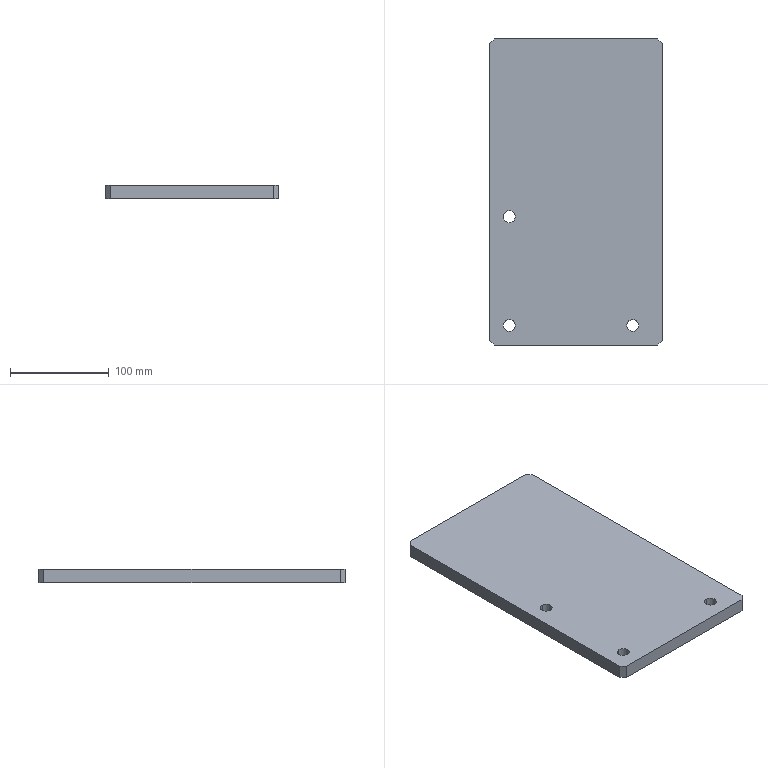Part | STEP file | [11] | 1 solid | 16 faces | box 175 x 310 x 14 mm | volume 754050 mm3 | plane 10 | cylinder 6 | commonest cylinder face diameters 12 x6
STEP:
#1=CARTESIAN_POINT('',(0.,0.,0.));
#2=DIRECTION('',(0.,0.,1.));
#3=DIRECTION('',(1.,0.,0.));
#4=AXIS2_PLACEMENT_3D('',#1,#2,#3);
#5=CARTESIAN_POINT('',(145.,26.,0.));
#6=VERTEX_POINT('',#5);
#7=CARTESIAN_POINT('',(145.,26.,14.));
#8=VERTEX_POINT('',#7);
#9=CARTESIAN_POINT('',(145.,26.,0.));
#10=DIRECTION('',(0.,0.,1.));
#11=VECTOR('',#10,1.);
#12=LINE('',#9,#11);
#13=CARTESIAN_POINT('',(145.,20.,0.));
#14=DIRECTION('',(0.,0.,1.));
#15=DIRECTION('',(0.,1.,0.));
#16=AXIS2_PLACEMENT_3D('',#13,#14,#15);
#17=CYLINDRICAL_SURFACE('',#16,6.);
#18=CARTESIAN_POINT('',(6.283,0.));
#19=DIRECTION('',(0.,1.));
#20=VECTOR('',#19,1.);
#21=LINE('',#18,#20);
#22=(GEOMETRIC_REPRESENTATION_CONTEXT(2)PARAMETRIC_REPRESENTATION_CONTEXT()REPRESENTATION_CONTEXT('',''));
#23=DEFINITIONAL_REPRESENTATION('',(#21),#22);
#24=PCURVE('',#17,#23);
#25=CARTESIAN_POINT('',(145.,20.,0.));
#26=DIRECTION('',(0.,0.,1.));
#27=DIRECTION('',(0.,1.,0.));
#28=AXIS2_PLACEMENT_3D('',#25,#26,#27);
#29=CYLINDRICAL_SURFACE('',#28,6.);
#30=CARTESIAN_POINT('',(0.,0.));
#31=DIRECTION('',(0.,1.));
#32=VECTOR('',#31,1.);
#33=LINE('',#30,#32);
#34=(GEOMETRIC_REPRESENTATION_CONTEXT(2)PARAMETRIC_REPRESENTATION_CONTEXT()REPRESENTATION_CONTEXT('',''));
#35=DEFINITIONAL_REPRESENTATION('',(#33),#34);
#36=PCURVE('',#29,#35);
#37=SURFACE_CURVE('',#12,(#24,#36),.PCURVE_S1.);
#38=EDGE_CURVE('',#6,#8,#37,.T.);
#39=ORIENTED_EDGE('',*,*,#38,.T.);
#40=CARTESIAN_POINT('',(145.,14.,14.));
#41=VERTEX_POINT('',#40);
#42=CARTESIAN_POINT('',(145.,20.,14.));
#43=DIRECTION('',(0.,0.,-1.));
#44=DIRECTION('',(0.,-1.,0.));
#45=AXIS2_PLACEMENT_3D('',#42,#43,#44);
#46=CIRCLE('',#45,6.);
#47=CARTESIAN_POINT('',(9.425,14.));
#48=DIRECTION('',(-1.,0.));
#49=VECTOR('',#48,1.);
#50=LINE('',#47,#49);
#51=(GEOMETRIC_REPRESENTATION_CONTEXT(2)PARAMETRIC_REPRESENTATION_CONTEXT()REPRESENTATION_CONTEXT('',''));
#52=DEFINITIONAL_REPRESENTATION('',(#50),#51);
#53=PCURVE('',#17,#52);
#54=CARTESIAN_POINT('',(87.5,155.,14.));
#55=DIRECTION('',(0.,0.,1.));
#56=DIRECTION('',(0.,1.,0.));
#57=AXIS2_PLACEMENT_3D('',#54,#55,#56);
#58=PLANE('',#57);
#59=CARTESIAN_POINT('',(-141.,-57.5));
#60=CARTESIAN_POINT('',(-141.,-47.108));
#61=CARTESIAN_POINT('',(-132.,-52.304));
#62=CARTESIAN_POINT('',(-123.,-57.5));
#63=CARTESIAN_POINT('',(-132.,-62.696));
#64=CARTESIAN_POINT('',(-141.,-67.892));
#65=CARTESIAN_POINT('',(-141.,-57.5));
#66=(BOUNDED_CURVE()B_SPLINE_CURVE(2,(#59,#60,#61,#62,#63,#64,#65),.UNSPECIFIED.,.T.,.F.)B_SPLINE_CURVE_WITH_KNOTS((1,2,2,2,2,1),(-2.094,0.,2.094,4.189,6.283,8.378),.UNSPECIFIED.)CURVE()GEOMETRIC_REPRESENTATION_ITEM()RATIONAL_B_SPLINE_CURVE((1.,0.5,1.,0.5,1.,0.5,1.))REPRESENTATION_ITEM(''));
#67=(GEOMETRIC_REPRESENTATION_CONTEXT(2)PARAMETRIC_REPRESENTATION_CONTEXT()REPRESENTATION_CONTEXT('',''));
#68=DEFINITIONAL_REPRESENTATION('',(#66),#67);
#69=PCURVE('',#58,#68);
#70=SURFACE_CURVE('',#46,(#53,#69),.PCURVE_S1.);
#71=EDGE_CURVE('',#8,#41,#70,.T.);
#72=ORIENTED_EDGE('',*,*,#71,.T.);
#73=CARTESIAN_POINT('',(145.,14.,0.));
#74=VERTEX_POINT('',#73);
#75=CARTESIAN_POINT('',(145.,14.,0.));
#76=DIRECTION('',(0.,0.,1.));
#77=VECTOR('',#76,1.);
#78=LINE('',#75,#77);
#79=CARTESIAN_POINT('',(3.142,0.));
#80=DIRECTION('',(0.,1.));
#81=VECTOR('',#80,1.);
#82=LINE('',#79,#81);
#83=(GEOMETRIC_REPRESENTATION_CONTEXT(2)PARAMETRIC_REPRESENTATION_CONTEXT()REPRESENTATION_CONTEXT('',''));
#84=DEFINITIONAL_REPRESENTATION('',(#82),#83);
#85=PCURVE('',#17,#84);
#86=CARTESIAN_POINT('',(3.142,0.));
#87=DIRECTION('',(0.,1.));
#88=VECTOR('',#87,1.);
#89=LINE('',#86,#88);
#90=(GEOMETRIC_REPRESENTATION_CONTEXT(2)PARAMETRIC_REPRESENTATION_CONTEXT()REPRESENTATION_CONTEXT('',''));
#91=DEFINITIONAL_REPRESENTATION('',(#89),#90);
#92=PCURVE('',#29,#91);
#93=SURFACE_CURVE('',#78,(#85,#92),.PCURVE_S1.);
#94=EDGE_CURVE('',#74,#41,#93,.T.);
#95=ORIENTED_EDGE('',*,*,#94,.F.);
#96=CARTESIAN_POINT('',(145.,20.,0.));
#97=DIRECTION('',(0.,0.,1.));
#98=DIRECTION('',(0.,1.,0.));
#99=AXIS2_PLACEMENT_3D('',#96,#97,#98);
#100=CIRCLE('',#99,6.);
#101=CARTESIAN_POINT('',(0.,0.));
#102=DIRECTION('',(1.,0.));
#103=VECTOR('',#102,1.);
#104=LINE('',#101,#103);
#105=(GEOMETRIC_REPRESENTATION_CONTEXT(2)PARAMETRIC_REPRESENTATION_CONTEXT()REPRESENTATION_CONTEXT('',''));
#106=DEFINITIONAL_REPRESENTATION('',(#104),#105);
#107=PCURVE('',#17,#106);
#108=CARTESIAN_POINT('',(87.5,155.,0.));
#109=DIRECTION('',(0.,0.,-1.));
#110=DIRECTION('',(0.,-1.,0.));
#111=AXIS2_PLACEMENT_3D('',#108,#109,#110);
#112=PLANE('',#111);
#113=CARTESIAN_POINT('',(129.,-57.5));
#114=CARTESIAN_POINT('',(129.,-47.108));
#115=CARTESIAN_POINT('',(138.,-52.304));
#116=CARTESIAN_POINT('',(147.,-57.5));
#117=CARTESIAN_POINT('',(138.,-62.696));
#118=CARTESIAN_POINT('',(129.,-67.892));
#119=CARTESIAN_POINT('',(129.,-57.5));
#120=(BOUNDED_CURVE()B_SPLINE_CURVE(2,(#113,#114,#115,#116,#117,#118,#119),.UNSPECIFIED.,.T.,.F.)B_SPLINE_CURVE_WITH_KNOTS((1,2,2,2,2,1),(-2.094,0.,2.094,4.189,6.283,8.378),.UNSPECIFIED.)CURVE()GEOMETRIC_REPRESENTATION_ITEM()RATIONAL_B_SPLINE_CURVE((1.,0.5,1.,0.5,1.,0.5,1.))REPRESENTATION_ITEM(''));
#121=(GEOMETRIC_REPRESENTATION_CONTEXT(2)PARAMETRIC_REPRESENTATION_CONTEXT()REPRESENTATION_CONTEXT('',''));
#122=DEFINITIONAL_REPRESENTATION('',(#120),#121);
#123=PCURVE('',#112,#122);
#124=SURFACE_CURVE('',#100,(#107,#123),.PCURVE_S1.);
#125=EDGE_CURVE('',#74,#6,#124,.T.);
#126=ORIENTED_EDGE('',*,*,#125,.T.);
#127=EDGE_LOOP('',(#39,#72,#95,#126));
#128=FACE_BOUND('',#127,.F.);
#129=ADVANCED_FACE('',(#128),#17,.F.);
#130=CARTESIAN_POINT('',(20.,136.,0.));
#131=VERTEX_POINT('',#130);
#132=CARTESIAN_POINT('',(20.,136.,14.));
#133=VERTEX_POINT('',#132);
#134=CARTESIAN_POINT('',(20.,136.,0.));
#135=DIRECTION('',(0.,0.,1.));
#136=VECTOR('',#135,1.);
#137=LINE('',#134,#136);
#138=CARTESIAN_POINT('',(20.,130.,0.));
#139=DIRECTION('',(0.,0.,1.));
#140=DIRECTION('',(0.,1.,0.));
#141=AXIS2_PLACEMENT_3D('',#138,#139,#140);
#142=CYLINDRICAL_SURFACE('',#141,6.);
#143=CARTESIAN_POINT('',(6.283,0.));
#144=DIRECTION('',(0.,1.));
#145=VECTOR('',#144,1.);
#146=LINE('',#143,#145);
#147=(GEOMETRIC_REPRESENTATION_CONTEXT(2)PARAMETRIC_REPRESENTATION_CONTEXT()REPRESENTATION_CONTEXT('',''));
#148=DEFINITIONAL_REPRESENTATION('',(#146),#147);
#149=PCURVE('',#142,#148);
#150=CARTESIAN_POINT('',(20.,130.,0.));
#151=DIRECTION('',(0.,0.,1.));
#152=DIRECTION('',(0.,1.,0.));
#153=AXIS2_PLACEMENT_3D('',#150,#151,#152);
#154=CYLINDRICAL_SURFACE('',#153,6.);
#155=CARTESIAN_POINT('',(0.,0.));
#156=DIRECTION('',(0.,1.));
#157=VECTOR('',#156,1.);
#158=LINE('',#155,#157);
#159=(GEOMETRIC_REPRESENTATION_CONTEXT(2)PARAMETRIC_REPRESENTATION_CONTEXT()REPRESENTATION_CONTEXT('',''));
#160=DEFINITIONAL_REPRESENTATION('',(#158),#159);
#161=PCURVE('',#154,#160);
#162=SURFACE_CURVE('',#137,(#149,#161),.PCURVE_S1.);
#163=EDGE_CURVE('',#131,#133,#162,.T.);
#164=ORIENTED_EDGE('',*,*,#163,.T.);
#165=CARTESIAN_POINT('',(20.,124.,14.));
#166=VERTEX_POINT('',#165);
#167=CARTESIAN_POINT('',(20.,130.,14.));
#168=DIRECTION('',(0.,0.,-1.));
#169=DIRECTION('',(0.,-1.,0.));
#170=AXIS2_PLACEMENT_3D('',#167,#168,#169);
#171=CIRCLE('',#170,6.);
#172=CARTESIAN_POINT('',(9.425,14.));
#173=DIRECTION('',(-1.,0.));
#174=VECTOR('',#173,1.);
#175=LINE('',#172,#174);
#176=(GEOMETRIC_REPRESENTATION_CONTEXT(2)PARAMETRIC_REPRESENTATION_CONTEXT()REPRESENTATION_CONTEXT('',''));
#177=DEFINITIONAL_REPRESENTATION('',(#175),#176);
#178=PCURVE('',#142,#177);
#179=CARTESIAN_POINT('',(-31.,67.5));
#180=CARTESIAN_POINT('',(-31.,77.892));
#181=CARTESIAN_POINT('',(-22.,72.696));
#182=CARTESIAN_POINT('',(-13.,67.5));
#183=CARTESIAN_POINT('',(-22.,62.304));
#184=CARTESIAN_POINT('',(-31.,57.108));
#185=CARTESIAN_POINT('',(-31.,67.5));
#186=(BOUNDED_CURVE()B_SPLINE_CURVE(2,(#179,#180,#181,#182,#183,#184,#185),.UNSPECIFIED.,.T.,.F.)B_SPLINE_CURVE_WITH_KNOTS((1,2,2,2,2,1),(-2.094,0.,2.094,4.189,6.283,8.378),.UNSPECIFIED.)CURVE()GEOMETRIC_REPRESENTATION_ITEM()RATIONAL_B_SPLINE_CURVE((1.,0.5,1.,0.5,1.,0.5,1.))REPRESENTATION_ITEM(''));
#187=(GEOMETRIC_REPRESENTATION_CONTEXT(2)PARAMETRIC_REPRESENTATION_CONTEXT()REPRESENTATION_CONTEXT('',''));
#188=DEFINITIONAL_REPRESENTATION('',(#186),#187);
#189=PCURVE('',#58,#188);
#190=SURFACE_CURVE('',#171,(#178,#189),.PCURVE_S1.);
#191=EDGE_CURVE('',#133,#166,#190,.T.);
#192=ORIENTED_EDGE('',*,*,#191,.T.);
#193=CARTESIAN_POINT('',(20.,124.,0.));
#194=VERTEX_POINT('',#193);
#195=CARTESIAN_POINT('',(20.,124.,0.));
#196=DIRECTION('',(0.,0.,1.));
#197=VECTOR('',#196,1.);
#198=LINE('',#195,#197);
#199=CARTESIAN_POINT('',(3.142,0.));
#200=DIRECTION('',(0.,1.));
#201=VECTOR('',#200,1.);
#202=LINE('',#199,#201);
#203=(GEOMETRIC_REPRESENTATION_CONTEXT(2)PARAMETRIC_REPRESENTATION_CONTEXT()REPRESENTATION_CONTEXT('',''));
#204=DEFINITIONAL_REPRESENTATION('',(#202),#203);
#205=PCURVE('',#142,#204);
#206=CARTESIAN_POINT('',(3.142,0.));
#207=DIRECTION('',(0.,1.));
#208=VECTOR('',#207,1.);
#209=LINE('',#206,#208);
#210=(GEOMETRIC_REPRESENTATION_CONTEXT(2)PARAMETRIC_REPRESENTATION_CONTEXT()REPRESENTATION_CONTEXT('',''));
#211=DEFINITIONAL_REPRESENTATION('',(#209),#210);
#212=PCURVE('',#154,#211);
#213=SURFACE_CURVE('',#198,(#205,#212),.PCURVE_S1.);
#214=EDGE_CURVE('',#194,#166,#213,.T.);
#215=ORIENTED_EDGE('',*,*,#214,.F.);
#216=CARTESIAN_POINT('',(20.,130.,0.));
#217=DIRECTION('',(0.,0.,1.));
#218=DIRECTION('',(0.,1.,0.));
#219=AXIS2_PLACEMENT_3D('',#216,#217,#218);
#220=CIRCLE('',#219,6.);
#221=CARTESIAN_POINT('',(0.,0.));
#222=DIRECTION('',(1.,0.));
#223=VECTOR('',#222,1.);
#224=LINE('',#221,#223);
#225=(GEOMETRIC_REPRESENTATION_CONTEXT(2)PARAMETRIC_REPRESENTATION_CONTEXT()REPRESENTATION_CONTEXT('',''));
#226=DEFINITIONAL_REPRESENTATION('',(#224),#225);
#227=PCURVE('',#142,#226);
#228=CARTESIAN_POINT('',(19.,67.5));
#229=CARTESIAN_POINT('',(19.,77.892));
#230=CARTESIAN_POINT('',(28.,72.696));
#231=CARTESIAN_POINT('',(37.,67.5));
#232=CARTESIAN_POINT('',(28.,62.304));
#233=CARTESIAN_POINT('',(19.,57.108));
#234=CARTESIAN_POINT('',(19.,67.5));
#235=(BOUNDED_CURVE()B_SPLINE_CURVE(2,(#228,#229,#230,#231,#232,#233,#234),.UNSPECIFIED.,.T.,.F.)B_SPLINE_CURVE_WITH_KNOTS((1,2,2,2,2,1),(-2.094,0.,2.094,4.189,6.283,8.378),.UNSPECIFIED.)CURVE()GEOMETRIC_REPRESENTATION_ITEM()RATIONAL_B_SPLINE_CURVE((1.,0.5,1.,0.5,1.,0.5,1.))REPRESENTATION_ITEM(''));
#236=(GEOMETRIC_REPRESENTATION_CONTEXT(2)PARAMETRIC_REPRESENTATION_CONTEXT()REPRESENTATION_CONTEXT('',''));
#237=DEFINITIONAL_REPRESENTATION('',(#235),#236);
#238=PCURVE('',#112,#237);
#239=SURFACE_CURVE('',#220,(#227,#238),.PCURVE_S1.);
#240=EDGE_CURVE('',#194,#131,#239,.T.);
#241=ORIENTED_EDGE('',*,*,#240,.T.);
#242=EDGE_LOOP('',(#164,#192,#215,#241));
#243=FACE_BOUND('',#242,.F.);
#244=ADVANCED_FACE('',(#243),#142,.F.);
#245=CARTESIAN_POINT('',(20.,26.,0.));
#246=VERTEX_POINT('',#245);
#247=CARTESIAN_POINT('',(20.,26.,14.));
#248=VERTEX_POINT('',#247);
#249=CARTESIAN_POINT('',(20.,26.,0.));
#250=DIRECTION('',(0.,0.,1.));
#251=VECTOR('',#250,1.);
#252=LINE('',#249,#251);
#253=CARTESIAN_POINT('',(20.,20.,0.));
#254=DIRECTION('',(0.,0.,1.));
#255=DIRECTION('',(0.,1.,0.));
#256=AXIS2_PLACEMENT_3D('',#253,#254,#255);
#257=CYLINDRICAL_SURFACE('',#256,6.);
#258=CARTESIAN_POINT('',(6.283,0.));
#259=DIRECTION('',(0.,1.));
#260=VECTOR('',#259,1.);
#261=LINE('',#258,#260);
#262=(GEOMETRIC_REPRESENTATION_CONTEXT(2)PARAMETRIC_REPRESENTATION_CONTEXT()REPRESENTATION_CONTEXT('',''));
#263=DEFINITIONAL_REPRESENTATION('',(#261),#262);
#264=PCURVE('',#257,#263);
#265=CARTESIAN_POINT('',(20.,20.,0.));
#266=DIRECTION('',(0.,0.,1.));
#267=DIRECTION('',(0.,1.,0.));
#268=AXIS2_PLACEMENT_3D('',#265,#266,#267);
#269=CYLINDRICAL_SURFACE('',#268,6.);
#270=CARTESIAN_POINT('',(0.,0.));
#271=DIRECTION('',(0.,1.));
#272=VECTOR('',#271,1.);
#273=LINE('',#270,#272);
#274=(GEOMETRIC_REPRESENTATION_CONTEXT(2)PARAMETRIC_REPRESENTATION_CONTEXT()REPRESENTATION_CONTEXT('',''));
#275=DEFINITIONAL_REPRESENTATION('',(#273),#274);
#276=PCURVE('',#269,#275);
#277=SURFACE_CURVE('',#252,(#264,#276),.PCURVE_S1.);
#278=EDGE_CURVE('',#246,#248,#277,.T.);
#279=ORIENTED_EDGE('',*,*,#278,.T.);
#280=CARTESIAN_POINT('',(20.,14.,14.));
#281=VERTEX_POINT('',#280);
#282=CARTESIAN_POINT('',(20.,20.,14.));
#283=DIRECTION('',(0.,0.,-1.));
#284=DIRECTION('',(0.,-1.,0.));
#285=AXIS2_PLACEMENT_3D('',#282,#283,#284);
#286=CIRCLE('',#285,6.);
#287=CARTESIAN_POINT('',(9.425,14.));
#288=DIRECTION('',(-1.,0.));
#289=VECTOR('',#288,1.);
#290=LINE('',#287,#289);
#291=(GEOMETRIC_REPRESENTATION_CONTEXT(2)PARAMETRIC_REPRESENTATION_CONTEXT()REPRESENTATION_CONTEXT('',''));
#292=DEFINITIONAL_REPRESENTATION('',(#290),#291);
#293=PCURVE('',#257,#292);
#294=CARTESIAN_POINT('',(-141.,67.5));
#295=CARTESIAN_POINT('',(-141.,77.892));
#296=CARTESIAN_POINT('',(-132.,72.696));
#297=CARTESIAN_POINT('',(-123.,67.5));
#298=CARTESIAN_POINT('',(-132.,62.304));
#299=CARTESIAN_POINT('',(-141.,57.108));
#300=CARTESIAN_POINT('',(-141.,67.5));
#301=(BOUNDED_CURVE()B_SPLINE_CURVE(2,(#294,#295,#296,#297,#298,#299,#300),.UNSPECIFIED.,.T.,.F.)B_SPLINE_CURVE_WITH_KNOTS((1,2,2,2,2,1),(-2.094,0.,2.094,4.189,6.283,8.378),.UNSPECIFIED.)CURVE()GEOMETRIC_REPRESENTATION_ITEM()RATIONAL_B_SPLINE_CURVE((1.,0.5,1.,0.5,1.,0.5,1.))REPRESENTATION_ITEM(''));
#302=(GEOMETRIC_REPRESENTATION_CONTEXT(2)PARAMETRIC_REPRESENTATION_CONTEXT()REPRESENTATION_CONTEXT('',''));
#303=DEFINITIONAL_REPRESENTATION('',(#301),#302);
#304=PCURVE('',#58,#303);
#305=SURFACE_CURVE('',#286,(#293,#304),.PCURVE_S1.);
#306=EDGE_CURVE('',#248,#281,#305,.T.);
#307=ORIENTED_EDGE('',*,*,#306,.T.);
#308=CARTESIAN_POINT('',(20.,14.,0.));
#309=VERTEX_POINT('',#308);
#310=CARTESIAN_POINT('',(20.,14.,0.));
#311=DIRECTION('',(0.,0.,1.));
#312=VECTOR('',#311,1.);
#313=LINE('',#310,#312);
#314=CARTESIAN_POINT('',(3.142,0.));
#315=DIRECTION('',(0.,1.));
#316=VECTOR('',#315,1.);
#317=LINE('',#314,#316);
#318=(GEOMETRIC_REPRESENTATION_CONTEXT(2)PARAMETRIC_REPRESENTATION_CONTEXT()REPRESENTATION_CONTEXT('',''));
#319=DEFINITIONAL_REPRESENTATION('',(#317),#318);
#320=PCURVE('',#257,#319);
#321=CARTESIAN_POINT('',(3.142,0.));
#322=DIRECTION('',(0.,1.));
#323=VECTOR('',#322,1.);
#324=LINE('',#321,#323);
#325=(GEOMETRIC_REPRESENTATION_CONTEXT(2)PARAMETRIC_REPRESENTATION_CONTEXT()REPRESENTATION_CONTEXT('',''));
#326=DEFINITIONAL_REPRESENTATION('',(#324),#325);
#327=PCURVE('',#269,#326);
#328=SURFACE_CURVE('',#313,(#320,#327),.PCURVE_S1.);
#329=EDGE_CURVE('',#309,#281,#328,.T.);
#330=ORIENTED_EDGE('',*,*,#329,.F.);
#331=CARTESIAN_POINT('',(20.,20.,0.));
#332=DIRECTION('',(0.,0.,1.));
#333=DIRECTION('',(0.,1.,0.));
#334=AXIS2_PLACEMENT_3D('',#331,#332,#333);
#335=CIRCLE('',#334,6.);
#336=CARTESIAN_POINT('',(0.,0.));
#337=DIRECTION('',(1.,0.));
#338=VECTOR('',#337,1.);
#339=LINE('',#336,#338);
#340=(GEOMETRIC_REPRESENTATION_CONTEXT(2)PARAMETRIC_REPRESENTATION_CONTEXT()REPRESENTATION_CONTEXT('',''));
#341=DEFINITIONAL_REPRESENTATION('',(#339),#340);
#342=PCURVE('',#257,#341);
#343=CARTESIAN_POINT('',(129.,67.5));
#344=CARTESIAN_POINT('',(129.,77.892));
#345=CARTESIAN_POINT('',(138.,72.696));
#346=CARTESIAN_POINT('',(147.,67.5));
#347=CARTESIAN_POINT('',(138.,62.304));
#348=CARTESIAN_POINT('',(129.,57.108));
#349=CARTESIAN_POINT('',(129.,67.5));
#350=(BOUNDED_CURVE()B_SPLINE_CURVE(2,(#343,#344,#345,#346,#347,#348,#349),.UNSPECIFIED.,.T.,.F.)B_SPLINE_CURVE_WITH_KNOTS((1,2,2,2,2,1),(-2.094,0.,2.094,4.189,6.283,8.378),.UNSPECIFIED.)CURVE()GEOMETRIC_REPRESENTATION_ITEM()RATIONAL_B_SPLINE_CURVE((1.,0.5,1.,0.5,1.,0.5,1.))REPRESENTATION_ITEM(''));
#351=(GEOMETRIC_REPRESENTATION_CONTEXT(2)PARAMETRIC_REPRESENTATION_CONTEXT()REPRESENTATION_CONTEXT('',''));
#352=DEFINITIONAL_REPRESENTATION('',(#350),#351);
#353=PCURVE('',#112,#352);
#354=SURFACE_CURVE('',#335,(#342,#353),.PCURVE_S1.);
#355=EDGE_CURVE('',#309,#246,#354,.T.);
#356=ORIENTED_EDGE('',*,*,#355,.T.);
#357=EDGE_LOOP('',(#279,#307,#330,#356));
#358=FACE_BOUND('',#357,.F.);
#359=ADVANCED_FACE('',(#358),#257,.F.);
#360=ORIENTED_EDGE('',*,*,#71,.T.);
#361=CARTESIAN_POINT('',(145.,20.,14.));
#362=DIRECTION('',(0.,0.,-1.));
#363=DIRECTION('',(0.,-1.,0.));
#364=AXIS2_PLACEMENT_3D('',#361,#362,#363);
#365=CIRCLE('',#364,6.);
#366=CARTESIAN_POINT('',(-141.,-57.5));
#367=CARTESIAN_POINT('',(-141.,-47.108));
#368=CARTESIAN_POINT('',(-132.,-52.304));
#369=CARTESIAN_POINT('',(-123.,-57.5));
#370=CARTESIAN_POINT('',(-132.,-62.696));
#371=CARTESIAN_POINT('',(-141.,-67.892));
#372=CARTESIAN_POINT('',(-141.,-57.5));
#373=(BOUNDED_CURVE()B_SPLINE_CURVE(2,(#366,#367,#368,#369,#370,#371,#372),.UNSPECIFIED.,.T.,.F.)B_SPLINE_CURVE_WITH_KNOTS((1,2,2,2,2,1),(-2.094,0.,2.094,4.189,6.283,8.378),.UNSPECIFIED.)CURVE()GEOMETRIC_REPRESENTATION_ITEM()RATIONAL_B_SPLINE_CURVE((1.,0.5,1.,0.5,1.,0.5,1.))REPRESENTATION_ITEM(''));
#374=(GEOMETRIC_REPRESENTATION_CONTEXT(2)PARAMETRIC_REPRESENTATION_CONTEXT()REPRESENTATION_CONTEXT('',''));
#375=DEFINITIONAL_REPRESENTATION('',(#373),#374);
#376=PCURVE('',#58,#375);
#377=CARTESIAN_POINT('',(3.142,14.));
#378=DIRECTION('',(-1.,0.));
#379=VECTOR('',#378,1.);
#380=LINE('',#377,#379);
#381=(GEOMETRIC_REPRESENTATION_CONTEXT(2)PARAMETRIC_REPRESENTATION_CONTEXT()REPRESENTATION_CONTEXT('',''));
#382=DEFINITIONAL_REPRESENTATION('',(#380),#381);
#383=PCURVE('',#29,#382);
#384=SURFACE_CURVE('',#365,(#376,#383),.PCURVE_S1.);
#385=EDGE_CURVE('',#41,#8,#384,.T.);
#386=ORIENTED_EDGE('',*,*,#385,.T.);
#387=EDGE_LOOP('',(#360,#386));
#388=FACE_BOUND('',#387,.T.);
#389=ORIENTED_EDGE('',*,*,#191,.T.);
#390=CARTESIAN_POINT('',(20.,130.,14.));
#391=DIRECTION('',(0.,0.,-1.));
#392=DIRECTION('',(0.,-1.,0.));
#393=AXIS2_PLACEMENT_3D('',#390,#391,#392);
#394=CIRCLE('',#393,6.);
#395=CARTESIAN_POINT('',(-31.,67.5));
#396=CARTESIAN_POINT('',(-31.,77.892));
#397=CARTESIAN_POINT('',(-22.,72.696));
#398=CARTESIAN_POINT('',(-13.,67.5));
#399=CARTESIAN_POINT('',(-22.,62.304));
#400=CARTESIAN_POINT('',(-31.,57.108));
#401=CARTESIAN_POINT('',(-31.,67.5));
#402=(BOUNDED_CURVE()B_SPLINE_CURVE(2,(#395,#396,#397,#398,#399,#400,#401),.UNSPECIFIED.,.T.,.F.)B_SPLINE_CURVE_WITH_KNOTS((1,2,2,2,2,1),(-2.094,0.,2.094,4.189,6.283,8.378),.UNSPECIFIED.)CURVE()GEOMETRIC_REPRESENTATION_ITEM()RATIONAL_B_SPLINE_CURVE((1.,0.5,1.,0.5,1.,0.5,1.))REPRESENTATION_ITEM(''));
#403=(GEOMETRIC_REPRESENTATION_CONTEXT(2)PARAMETRIC_REPRESENTATION_CONTEXT()REPRESENTATION_CONTEXT('',''));
#404=DEFINITIONAL_REPRESENTATION('',(#402),#403);
#405=PCURVE('',#58,#404);
#406=CARTESIAN_POINT('',(3.142,14.));
#407=DIRECTION('',(-1.,0.));
#408=VECTOR('',#407,1.);
#409=LINE('',#406,#408);
#410=(GEOMETRIC_REPRESENTATION_CONTEXT(2)PARAMETRIC_REPRESENTATION_CONTEXT()REPRESENTATION_CONTEXT('',''));
#411=DEFINITIONAL_REPRESENTATION('',(#409),#410);
#412=PCURVE('',#154,#411);
#413=SURFACE_CURVE('',#394,(#405,#412),.PCURVE_S1.);
#414=EDGE_CURVE('',#166,#133,#413,.T.);
#415=ORIENTED_EDGE('',*,*,#414,.T.);
#416=EDGE_LOOP('',(#389,#415));
#417=FACE_BOUND('',#416,.T.);
#418=ORIENTED_EDGE('',*,*,#306,.T.);
#419=CARTESIAN_POINT('',(20.,20.,14.));
#420=DIRECTION('',(0.,0.,-1.));
#421=DIRECTION('',(0.,-1.,0.));
#422=AXIS2_PLACEMENT_3D('',#419,#420,#421);
#423=CIRCLE('',#422,6.);
#424=CARTESIAN_POINT('',(-141.,67.5));
#425=CARTESIAN_POINT('',(-141.,77.892));
#426=CARTESIAN_POINT('',(-132.,72.696));
#427=CARTESIAN_POINT('',(-123.,67.5));
#428=CARTESIAN_POINT('',(-132.,62.304));
#429=CARTESIAN_POINT('',(-141.,57.108));
#430=CARTESIAN_POINT('',(-141.,67.5));
#431=(BOUNDED_CURVE()B_SPLINE_CURVE(2,(#424,#425,#426,#427,#428,#429,#430),.UNSPECIFIED.,.T.,.F.)B_SPLINE_CURVE_WITH_KNOTS((1,2,2,2,2,1),(-2.094,0.,2.094,4.189,6.283,8.378),.UNSPECIFIED.)CURVE()GEOMETRIC_REPRESENTATION_ITEM()RATIONAL_B_SPLINE_CURVE((1.,0.5,1.,0.5,1.,0.5,1.))REPRESENTATION_ITEM(''));
#432=(GEOMETRIC_REPRESENTATION_CONTEXT(2)PARAMETRIC_REPRESENTATION_CONTEXT()REPRESENTATION_CONTEXT('',''));
#433=DEFINITIONAL_REPRESENTATION('',(#431),#432);
#434=PCURVE('',#58,#433);
#435=CARTESIAN_POINT('',(3.142,14.));
#436=DIRECTION('',(-1.,0.));
#437=VECTOR('',#436,1.);
#438=LINE('',#435,#437);
#439=(GEOMETRIC_REPRESENTATION_CONTEXT(2)PARAMETRIC_REPRESENTATION_CONTEXT()REPRESENTATION_CONTEXT('',''));
#440=DEFINITIONAL_REPRESENTATION('',(#438),#439);
#441=PCURVE('',#269,#440);
#442=SURFACE_CURVE('',#423,(#434,#441),.PCURVE_S1.);
#443=EDGE_CURVE('',#281,#248,#442,.T.);
#444=ORIENTED_EDGE('',*,*,#443,.T.);
#445=EDGE_LOOP('',(#418,#444));
#446=FACE_BOUND('',#445,.T.);
#447=CARTESIAN_POINT('',(5.,310.,14.));
#448=VERTEX_POINT('',#447);
#449=CARTESIAN_POINT('',(170.,310.,14.));
#450=VERTEX_POINT('',#449);
#451=CARTESIAN_POINT('',(87.5,310.,14.));
#452=DIRECTION('',(1.,0.,0.));
#453=VECTOR('',#452,1.);
#454=LINE('',#451,#453);
#455=CARTESIAN_POINT('',(155.,0.));
#456=DIRECTION('',(0.,-1.));
#457=VECTOR('',#456,1.);
#458=LINE('',#455,#457);
#459=(GEOMETRIC_REPRESENTATION_CONTEXT(2)PARAMETRIC_REPRESENTATION_CONTEXT()REPRESENTATION_CONTEXT('',''));
#460=DEFINITIONAL_REPRESENTATION('',(#458),#459);
#461=PCURVE('',#58,#460);
#462=CARTESIAN_POINT('',(87.5,310.,0.));
#463=DIRECTION('',(0.,1.,0.));
#464=DIRECTION('',(0.,0.,-1.));
#465=AXIS2_PLACEMENT_3D('',#462,#463,#464);
#466=PLANE('',#465);
#467=CARTESIAN_POINT('',(-14.,0.));
#468=DIRECTION('',(0.,-1.));
#469=VECTOR('',#468,1.);
#470=LINE('',#467,#469);
#471=(GEOMETRIC_REPRESENTATION_CONTEXT(2)PARAMETRIC_REPRESENTATION_CONTEXT()REPRESENTATION_CONTEXT('',''));
#472=DEFINITIONAL_REPRESENTATION('',(#470),#471);
#473=PCURVE('',#466,#472);
#474=SURFACE_CURVE('',#454,(#461,#473),.PCURVE_S1.);
#475=EDGE_CURVE('',#448,#450,#474,.T.);
#476=ORIENTED_EDGE('',*,*,#475,.F.);
#477=CARTESIAN_POINT('',(0.,305.,14.));
#478=VERTEX_POINT('',#477);
#479=CARTESIAN_POINT('',(-31.25,273.75,14.));
#480=DIRECTION('',(-0.7071,-0.7071,0.));
#481=VECTOR('',#480,1.);
#482=LINE('',#479,#481);
#483=CARTESIAN_POINT('',(118.75,118.75));
#484=DIRECTION('',(-0.7071,0.7071));
#485=VECTOR('',#484,1.);
#486=LINE('',#483,#485);
#487=(GEOMETRIC_REPRESENTATION_CONTEXT(2)PARAMETRIC_REPRESENTATION_CONTEXT()REPRESENTATION_CONTEXT('',''));
#488=DEFINITIONAL_REPRESENTATION('',(#486),#487);
#489=PCURVE('',#58,#488);
#490=CARTESIAN_POINT('',(5.,310.,0.));
#491=DIRECTION('',(0.7071,-0.7071,0.));
#492=DIRECTION('',(0.,0.,1.));
#493=AXIS2_PLACEMENT_3D('',#490,#491,#492);
#494=PLANE('',#493);
#495=CARTESIAN_POINT('',(14.,51.265));
#496=DIRECTION('',(0.,1.));
#497=VECTOR('',#496,1.);
#498=LINE('',#495,#497);
#499=(GEOMETRIC_REPRESENTATION_CONTEXT(2)PARAMETRIC_REPRESENTATION_CONTEXT()REPRESENTATION_CONTEXT('',''));
#500=DEFINITIONAL_REPRESENTATION('',(#498),#499);
#501=PCURVE('',#494,#500);
#502=SURFACE_CURVE('',#482,(#489,#501),.PCURVE_S1.);
#503=EDGE_CURVE('',#448,#478,#502,.T.);
#504=ORIENTED_EDGE('',*,*,#503,.T.);
#505=CARTESIAN_POINT('',(0.,5.,14.));
#506=VERTEX_POINT('',#505);
#507=CARTESIAN_POINT('',(0.,155.,14.));
#508=DIRECTION('',(0.,1.,0.));
#509=VECTOR('',#508,1.);
#510=LINE('',#507,#509);
#511=CARTESIAN_POINT('',(0.,87.5));
#512=DIRECTION('',(1.,0.));
#513=VECTOR('',#512,1.);
#514=LINE('',#511,#513);
#515=(GEOMETRIC_REPRESENTATION_CONTEXT(2)PARAMETRIC_REPRESENTATION_CONTEXT()REPRESENTATION_CONTEXT('',''));
#516=DEFINITIONAL_REPRESENTATION('',(#514),#515);
#517=PCURVE('',#58,#516);
#518=CARTESIAN_POINT('',(0.,155.,0.));
#519=DIRECTION('',(-1.,0.,0.));
#520=DIRECTION('',(0.,0.,1.));
#521=AXIS2_PLACEMENT_3D('',#518,#519,#520);
#522=PLANE('',#521);
#523=CARTESIAN_POINT('',(14.,0.));
#524=DIRECTION('',(0.,1.));
#525=VECTOR('',#524,1.);
#526=LINE('',#523,#525);
#527=(GEOMETRIC_REPRESENTATION_CONTEXT(2)PARAMETRIC_REPRESENTATION_CONTEXT()REPRESENTATION_CONTEXT('',''));
#528=DEFINITIONAL_REPRESENTATION('',(#526),#527);
#529=PCURVE('',#522,#528);
#530=SURFACE_CURVE('',#510,(#517,#529),.PCURVE_S1.);
#531=EDGE_CURVE('',#506,#478,#530,.T.);
#532=ORIENTED_EDGE('',*,*,#531,.F.);
#533=CARTESIAN_POINT('',(5.,0.,14.));
#534=VERTEX_POINT('',#533);
#535=CARTESIAN_POINT('',(-31.25,36.25,14.));
#536=DIRECTION('',(0.7071,-0.7071,0.));
#537=VECTOR('',#536,1.);
#538=LINE('',#535,#537);
#539=CARTESIAN_POINT('',(-118.75,118.75));
#540=DIRECTION('',(-0.7071,-0.7071));
#541=VECTOR('',#540,1.);
#542=LINE('',#539,#541);
#543=(GEOMETRIC_REPRESENTATION_CONTEXT(2)PARAMETRIC_REPRESENTATION_CONTEXT()REPRESENTATION_CONTEXT('',''));
#544=DEFINITIONAL_REPRESENTATION('',(#542),#543);
#545=PCURVE('',#58,#544);
#546=CARTESIAN_POINT('',(0.,5.,0.));
#547=DIRECTION('',(0.7071,0.7071,0.));
#548=DIRECTION('',(0.,0.,1.));
#549=AXIS2_PLACEMENT_3D('',#546,#547,#548);
#550=PLANE('',#549);
#551=CARTESIAN_POINT('',(14.,-44.194));
#552=DIRECTION('',(0.,1.));
#553=VECTOR('',#552,1.);
#554=LINE('',#551,#553);
#555=(GEOMETRIC_REPRESENTATION_CONTEXT(2)PARAMETRIC_REPRESENTATION_CONTEXT()REPRESENTATION_CONTEXT('',''));
#556=DEFINITIONAL_REPRESENTATION('',(#554),#555);
#557=PCURVE('',#550,#556);
#558=SURFACE_CURVE('',#538,(#545,#557),.PCURVE_S1.);
#559=EDGE_CURVE('',#506,#534,#558,.T.);
#560=ORIENTED_EDGE('',*,*,#559,.T.);
#561=CARTESIAN_POINT('',(170.,0.,14.));
#562=VERTEX_POINT('',#561);
#563=CARTESIAN_POINT('',(87.5,0.,14.));
#564=DIRECTION('',(-1.,0.,0.));
#565=VECTOR('',#564,1.);
#566=LINE('',#563,#565);
#567=CARTESIAN_POINT('',(-155.,0.));
#568=DIRECTION('',(0.,1.));
#569=VECTOR('',#568,1.);
#570=LINE('',#567,#569);
#571=(GEOMETRIC_REPRESENTATION_CONTEXT(2)PARAMETRIC_REPRESENTATION_CONTEXT()REPRESENTATION_CONTEXT('',''));
#572=DEFINITIONAL_REPRESENTATION('',(#570),#571);
#573=PCURVE('',#58,#572);
#574=CARTESIAN_POINT('',(87.5,0.,0.));
#575=DIRECTION('',(0.,-1.,0.));
#576=DIRECTION('',(0.,0.,1.));
#577=AXIS2_PLACEMENT_3D('',#574,#575,#576);
#578=PLANE('',#577);
#579=CARTESIAN_POINT('',(14.,0.));
#580=DIRECTION('',(0.,1.));
#581=VECTOR('',#580,1.);
#582=LINE('',#579,#581);
#583=(GEOMETRIC_REPRESENTATION_CONTEXT(2)PARAMETRIC_REPRESENTATION_CONTEXT()REPRESENTATION_CONTEXT('',''));
#584=DEFINITIONAL_REPRESENTATION('',(#582),#583);
#585=PCURVE('',#578,#584);
#586=SURFACE_CURVE('',#566,(#573,#585),.PCURVE_S1.);
#587=EDGE_CURVE('',#562,#534,#586,.T.);
#588=ORIENTED_EDGE('',*,*,#587,.F.);
#589=CARTESIAN_POINT('',(175.,5.,14.));
#590=VERTEX_POINT('',#589);
#591=CARTESIAN_POINT('',(206.25,36.25,14.));
#592=DIRECTION('',(0.7071,0.7071,0.));
#593=VECTOR('',#592,1.);
#594=LINE('',#591,#593);
#595=CARTESIAN_POINT('',(-118.75,-118.75));
#596=DIRECTION('',(0.7071,-0.7071));
#597=VECTOR('',#596,1.);
#598=LINE('',#595,#597);
#599=(GEOMETRIC_REPRESENTATION_CONTEXT(2)PARAMETRIC_REPRESENTATION_CONTEXT()REPRESENTATION_CONTEXT('',''));
#600=DEFINITIONAL_REPRESENTATION('',(#598),#599);
#601=PCURVE('',#58,#600);
#602=CARTESIAN_POINT('',(170.,0.,0.));
#603=DIRECTION('',(-0.7071,0.7071,0.));
#604=DIRECTION('',(0.,0.,1.));
#605=AXIS2_PLACEMENT_3D('',#602,#603,#604);
#606=PLANE('',#605);
#607=CARTESIAN_POINT('',(14.,51.265));
#608=DIRECTION('',(0.,1.));
#609=VECTOR('',#608,1.);
#610=LINE('',#607,#609);
#611=(GEOMETRIC_REPRESENTATION_CONTEXT(2)PARAMETRIC_REPRESENTATION_CONTEXT()REPRESENTATION_CONTEXT('',''));
#612=DEFINITIONAL_REPRESENTATION('',(#610),#611);
#613=PCURVE('',#606,#612);
#614=SURFACE_CURVE('',#594,(#601,#613),.PCURVE_S1.);
#615=EDGE_CURVE('',#562,#590,#614,.T.);
#616=ORIENTED_EDGE('',*,*,#615,.T.);
#617=CARTESIAN_POINT('',(175.,305.,14.));
#618=VERTEX_POINT('',#617);
#619=CARTESIAN_POINT('',(175.,155.,14.));
#620=DIRECTION('',(0.,-1.,0.));
#621=VECTOR('',#620,1.);
#622=LINE('',#619,#621);
#623=CARTESIAN_POINT('',(0.,-87.5));
#624=DIRECTION('',(-1.,0.));
#625=VECTOR('',#624,1.);
#626=LINE('',#623,#625);
#627=(GEOMETRIC_REPRESENTATION_CONTEXT(2)PARAMETRIC_REPRESENTATION_CONTEXT()REPRESENTATION_CONTEXT('',''));
#628=DEFINITIONAL_REPRESENTATION('',(#626),#627);
#629=PCURVE('',#58,#628);
#630=CARTESIAN_POINT('',(175.,155.,0.));
#631=DIRECTION('',(1.,0.,0.));
#632=DIRECTION('',(0.,0.,-1.));
#633=AXIS2_PLACEMENT_3D('',#630,#631,#632);
#634=PLANE('',#633);
#635=CARTESIAN_POINT('',(-14.,0.));
#636=DIRECTION('',(0.,-1.));
#637=VECTOR('',#636,1.);
#638=LINE('',#635,#637);
#639=(GEOMETRIC_REPRESENTATION_CONTEXT(2)PARAMETRIC_REPRESENTATION_CONTEXT()REPRESENTATION_CONTEXT('',''));
#640=DEFINITIONAL_REPRESENTATION('',(#638),#639);
#641=PCURVE('',#634,#640);
#642=SURFACE_CURVE('',#622,(#629,#641),.PCURVE_S1.);
#643=EDGE_CURVE('',#618,#590,#642,.T.);
#644=ORIENTED_EDGE('',*,*,#643,.F.);
#645=CARTESIAN_POINT('',(206.25,273.75,14.));
#646=DIRECTION('',(-0.7071,0.7071,0.));
#647=VECTOR('',#646,1.);
#648=LINE('',#645,#647);
#649=CARTESIAN_POINT('',(118.75,-118.75));
#650=DIRECTION('',(0.7071,0.7071));
#651=VECTOR('',#650,1.);
#652=LINE('',#649,#651);
#653=(GEOMETRIC_REPRESENTATION_CONTEXT(2)PARAMETRIC_REPRESENTATION_CONTEXT()REPRESENTATION_CONTEXT('',''));
#654=DEFINITIONAL_REPRESENTATION('',(#652),#653);
#655=PCURVE('',#58,#654);
#656=CARTESIAN_POINT('',(175.,305.,0.));
#657=DIRECTION('',(-0.7071,-0.7071,0.));
#658=DIRECTION('',(0.,0.,1.));
#659=AXIS2_PLACEMENT_3D('',#656,#657,#658);
#660=PLANE('',#659);
#661=CARTESIAN_POINT('',(14.,-44.194));
#662=DIRECTION('',(0.,1.));
#663=VECTOR('',#662,1.);
#664=LINE('',#661,#663);
#665=(GEOMETRIC_REPRESENTATION_CONTEXT(2)PARAMETRIC_REPRESENTATION_CONTEXT()REPRESENTATION_CONTEXT('',''));
#666=DEFINITIONAL_REPRESENTATION('',(#664),#665);
#667=PCURVE('',#660,#666);
#668=SURFACE_CURVE('',#648,(#655,#667),.PCURVE_S1.);
#669=EDGE_CURVE('',#618,#450,#668,.T.);
#670=ORIENTED_EDGE('',*,*,#669,.T.);
#671=EDGE_LOOP('',(#476,#504,#532,#560,#588,#616,#644,#670));
#672=FACE_BOUND('',#671,.T.);
#673=ADVANCED_FACE('',(#388,#417,#446,#672),#58,.T.);
#674=ORIENTED_EDGE('',*,*,#643,.T.);
#675=CARTESIAN_POINT('',(175.,5.,0.));
#676=VERTEX_POINT('',#675);
#677=CARTESIAN_POINT('',(175.,5.,0.));
#678=DIRECTION('',(0.,0.,-1.));
#679=VECTOR('',#678,1.);
#680=LINE('',#677,#679);
#681=CARTESIAN_POINT('',(0.,-150.));
#682=DIRECTION('',(1.,0.));
#683=VECTOR('',#682,1.);
#684=LINE('',#681,#683);
#685=(GEOMETRIC_REPRESENTATION_CONTEXT(2)PARAMETRIC_REPRESENTATION_CONTEXT()REPRESENTATION_CONTEXT('',''));
#686=DEFINITIONAL_REPRESENTATION('',(#684),#685);
#687=PCURVE('',#634,#686);
#688=CARTESIAN_POINT('',(0.,7.071));
#689=DIRECTION('',(-1.,0.));
#690=VECTOR('',#689,1.);
#691=LINE('',#688,#690);
#692=(GEOMETRIC_REPRESENTATION_CONTEXT(2)PARAMETRIC_REPRESENTATION_CONTEXT()REPRESENTATION_CONTEXT('',''));
#693=DEFINITIONAL_REPRESENTATION('',(#691),#692);
#694=PCURVE('',#606,#693);
#695=SURFACE_CURVE('',#680,(#687,#694),.PCURVE_S1.);
#696=EDGE_CURVE('',#590,#676,#695,.T.);
#697=ORIENTED_EDGE('',*,*,#696,.T.);
#698=CARTESIAN_POINT('',(175.,305.,0.));
#699=VERTEX_POINT('',#698);
#700=CARTESIAN_POINT('',(175.,155.,0.));
#701=DIRECTION('',(0.,1.,0.));
#702=VECTOR('',#701,1.);
#703=LINE('',#700,#702);
#704=CARTESIAN_POINT('',(0.,0.));
#705=DIRECTION('',(0.,1.));
#706=VECTOR('',#705,1.);
#707=LINE('',#704,#706);
#708=(GEOMETRIC_REPRESENTATION_CONTEXT(2)PARAMETRIC_REPRESENTATION_CONTEXT()REPRESENTATION_CONTEXT('',''));
#709=DEFINITIONAL_REPRESENTATION('',(#707),#708);
#710=PCURVE('',#634,#709);
#711=CARTESIAN_POINT('',(0.,-87.5));
#712=DIRECTION('',(-1.,0.));
#713=VECTOR('',#712,1.);
#714=LINE('',#711,#713);
#715=(GEOMETRIC_REPRESENTATION_CONTEXT(2)PARAMETRIC_REPRESENTATION_CONTEXT()REPRESENTATION_CONTEXT('',''));
#716=DEFINITIONAL_REPRESENTATION('',(#714),#715);
#717=PCURVE('',#112,#716);
#718=SURFACE_CURVE('',#703,(#710,#717),.PCURVE_S1.);
#719=EDGE_CURVE('',#676,#699,#718,.T.);
#720=ORIENTED_EDGE('',*,*,#719,.T.);
#721=CARTESIAN_POINT('',(175.,305.,0.));
#722=DIRECTION('',(0.,0.,1.));
#723=VECTOR('',#722,1.);
#724=LINE('',#721,#723);
#725=CARTESIAN_POINT('',(0.,150.));
#726=DIRECTION('',(-1.,0.));
#727=VECTOR('',#726,1.);
#728=LINE('',#725,#727);
#729=(GEOMETRIC_REPRESENTATION_CONTEXT(2)PARAMETRIC_REPRESENTATION_CONTEXT()REPRESENTATION_CONTEXT('',''));
#730=DEFINITIONAL_REPRESENTATION('',(#728),#729);
#731=PCURVE('',#634,#730);
#732=CARTESIAN_POINT('',(0.,0.));
#733=DIRECTION('',(1.,0.));
#734=VECTOR('',#733,1.);
#735=LINE('',#732,#734);
#736=(GEOMETRIC_REPRESENTATION_CONTEXT(2)PARAMETRIC_REPRESENTATION_CONTEXT()REPRESENTATION_CONTEXT('',''));
#737=DEFINITIONAL_REPRESENTATION('',(#735),#736);
#738=PCURVE('',#660,#737);
#739=SURFACE_CURVE('',#724,(#731,#738),.PCURVE_S1.);
#740=EDGE_CURVE('',#699,#618,#739,.T.);
#741=ORIENTED_EDGE('',*,*,#740,.T.);
#742=EDGE_LOOP('',(#674,#697,#720,#741));
#743=FACE_BOUND('',#742,.T.);
#744=ADVANCED_FACE('',(#743),#634,.T.);
#745=ORIENTED_EDGE('',*,*,#587,.T.);
#746=CARTESIAN_POINT('',(5.,0.,0.));
#747=VERTEX_POINT('',#746);
#748=CARTESIAN_POINT('',(5.,0.,0.));
#749=DIRECTION('',(0.,0.,-1.));
#750=VECTOR('',#749,1.);
#751=LINE('',#748,#750);
#752=CARTESIAN_POINT('',(0.,82.5));
#753=DIRECTION('',(-1.,0.));
#754=VECTOR('',#753,1.);
#755=LINE('',#752,#754);
#756=(GEOMETRIC_REPRESENTATION_CONTEXT(2)PARAMETRIC_REPRESENTATION_CONTEXT()REPRESENTATION_CONTEXT('',''));
#757=DEFINITIONAL_REPRESENTATION('',(#755),#756);
#758=PCURVE('',#578,#757);
#759=CARTESIAN_POINT('',(0.,7.071));
#760=DIRECTION('',(-1.,0.));
#761=VECTOR('',#760,1.);
#762=LINE('',#759,#761);
#763=(GEOMETRIC_REPRESENTATION_CONTEXT(2)PARAMETRIC_REPRESENTATION_CONTEXT()REPRESENTATION_CONTEXT('',''));
#764=DEFINITIONAL_REPRESENTATION('',(#762),#763);
#765=PCURVE('',#550,#764);
#766=SURFACE_CURVE('',#751,(#758,#765),.PCURVE_S1.);
#767=EDGE_CURVE('',#534,#747,#766,.T.);
#768=ORIENTED_EDGE('',*,*,#767,.T.);
#769=CARTESIAN_POINT('',(170.,0.,0.));
#770=VERTEX_POINT('',#769);
#771=CARTESIAN_POINT('',(87.5,0.,0.));
#772=DIRECTION('',(1.,0.,0.));
#773=VECTOR('',#772,1.);
#774=LINE('',#771,#773);
#775=CARTESIAN_POINT('',(0.,0.));
#776=DIRECTION('',(0.,-1.));
#777=VECTOR('',#776,1.);
#778=LINE('',#775,#777);
#779=(GEOMETRIC_REPRESENTATION_CONTEXT(2)PARAMETRIC_REPRESENTATION_CONTEXT()REPRESENTATION_CONTEXT('',''));
#780=DEFINITIONAL_REPRESENTATION('',(#778),#779);
#781=PCURVE('',#578,#780);
#782=CARTESIAN_POINT('',(155.,0.));
#783=DIRECTION('',(0.,-1.));
#784=VECTOR('',#783,1.);
#785=LINE('',#782,#784);
#786=(GEOMETRIC_REPRESENTATION_CONTEXT(2)PARAMETRIC_REPRESENTATION_CONTEXT()REPRESENTATION_CONTEXT('',''));
#787=DEFINITIONAL_REPRESENTATION('',(#785),#786);
#788=PCURVE('',#112,#787);
#789=SURFACE_CURVE('',#774,(#781,#788),.PCURVE_S1.);
#790=EDGE_CURVE('',#747,#770,#789,.T.);
#791=ORIENTED_EDGE('',*,*,#790,.T.);
#792=CARTESIAN_POINT('',(170.,0.,0.));
#793=DIRECTION('',(0.,0.,1.));
#794=VECTOR('',#793,1.);
#795=LINE('',#792,#794);
#796=CARTESIAN_POINT('',(0.,-82.5));
#797=DIRECTION('',(1.,0.));
#798=VECTOR('',#797,1.);
#799=LINE('',#796,#798);
#800=(GEOMETRIC_REPRESENTATION_CONTEXT(2)PARAMETRIC_REPRESENTATION_CONTEXT()REPRESENTATION_CONTEXT('',''));
#801=DEFINITIONAL_REPRESENTATION('',(#799),#800);
#802=PCURVE('',#578,#801);
#803=CARTESIAN_POINT('',(0.,0.));
#804=DIRECTION('',(1.,0.));
#805=VECTOR('',#804,1.);
#806=LINE('',#803,#805);
#807=(GEOMETRIC_REPRESENTATION_CONTEXT(2)PARAMETRIC_REPRESENTATION_CONTEXT()REPRESENTATION_CONTEXT('',''));
#808=DEFINITIONAL_REPRESENTATION('',(#806),#807);
#809=PCURVE('',#606,#808);
#810=SURFACE_CURVE('',#795,(#802,#809),.PCURVE_S1.);
#811=EDGE_CURVE('',#770,#562,#810,.T.);
#812=ORIENTED_EDGE('',*,*,#811,.T.);
#813=EDGE_LOOP('',(#745,#768,#791,#812));
#814=FACE_BOUND('',#813,.T.);
#815=ADVANCED_FACE('',(#814),#578,.T.);
#816=ORIENTED_EDGE('',*,*,#531,.T.);
#817=CARTESIAN_POINT('',(0.,305.,0.));
#818=VERTEX_POINT('',#817);
#819=CARTESIAN_POINT('',(0.,305.,0.));
#820=DIRECTION('',(0.,0.,-1.));
#821=VECTOR('',#820,1.);
#822=LINE('',#819,#821);
#823=CARTESIAN_POINT('',(0.,150.));
#824=DIRECTION('',(-1.,0.));
#825=VECTOR('',#824,1.);
#826=LINE('',#823,#825);
#827=(GEOMETRIC_REPRESENTATION_CONTEXT(2)PARAMETRIC_REPRESENTATION_CONTEXT()REPRESENTATION_CONTEXT('',''));
#828=DEFINITIONAL_REPRESENTATION('',(#826),#827);
#829=PCURVE('',#522,#828);
#830=CARTESIAN_POINT('',(0.,7.071));
#831=DIRECTION('',(-1.,0.));
#832=VECTOR('',#831,1.);
#833=LINE('',#830,#832);
#834=(GEOMETRIC_REPRESENTATION_CONTEXT(2)PARAMETRIC_REPRESENTATION_CONTEXT()REPRESENTATION_CONTEXT('',''));
#835=DEFINITIONAL_REPRESENTATION('',(#833),#834);
#836=PCURVE('',#494,#835);
#837=SURFACE_CURVE('',#822,(#829,#836),.PCURVE_S1.);
#838=EDGE_CURVE('',#478,#818,#837,.T.);
#839=ORIENTED_EDGE('',*,*,#838,.T.);
#840=CARTESIAN_POINT('',(0.,5.,0.));
#841=VERTEX_POINT('',#840);
#842=CARTESIAN_POINT('',(0.,155.,0.));
#843=DIRECTION('',(0.,-1.,0.));
#844=VECTOR('',#843,1.);
#845=LINE('',#842,#844);
#846=CARTESIAN_POINT('',(0.,0.));
#847=DIRECTION('',(0.,-1.));
#848=VECTOR('',#847,1.);
#849=LINE('',#846,#848);
#850=(GEOMETRIC_REPRESENTATION_CONTEXT(2)PARAMETRIC_REPRESENTATION_CONTEXT()REPRESENTATION_CONTEXT('',''));
#851=DEFINITIONAL_REPRESENTATION('',(#849),#850);
#852=PCURVE('',#522,#851);
#853=CARTESIAN_POINT('',(0.,87.5));
#854=DIRECTION('',(1.,0.));
#855=VECTOR('',#854,1.);
#856=LINE('',#853,#855);
#857=(GEOMETRIC_REPRESENTATION_CONTEXT(2)PARAMETRIC_REPRESENTATION_CONTEXT()REPRESENTATION_CONTEXT('',''));
#858=DEFINITIONAL_REPRESENTATION('',(#856),#857);
#859=PCURVE('',#112,#858);
#860=SURFACE_CURVE('',#845,(#852,#859),.PCURVE_S1.);
#861=EDGE_CURVE('',#818,#841,#860,.T.);
#862=ORIENTED_EDGE('',*,*,#861,.T.);
#863=CARTESIAN_POINT('',(0.,5.,0.));
#864=DIRECTION('',(0.,0.,1.));
#865=VECTOR('',#864,1.);
#866=LINE('',#863,#865);
#867=CARTESIAN_POINT('',(0.,-150.));
#868=DIRECTION('',(1.,0.));
#869=VECTOR('',#868,1.);
#870=LINE('',#867,#869);
#871=(GEOMETRIC_REPRESENTATION_CONTEXT(2)PARAMETRIC_REPRESENTATION_CONTEXT()REPRESENTATION_CONTEXT('',''));
#872=DEFINITIONAL_REPRESENTATION('',(#870),#871);
#873=PCURVE('',#522,#872);
#874=CARTESIAN_POINT('',(0.,0.));
#875=DIRECTION('',(1.,0.));
#876=VECTOR('',#875,1.);
#877=LINE('',#874,#876);
#878=(GEOMETRIC_REPRESENTATION_CONTEXT(2)PARAMETRIC_REPRESENTATION_CONTEXT()REPRESENTATION_CONTEXT('',''));
#879=DEFINITIONAL_REPRESENTATION('',(#877),#878);
#880=PCURVE('',#550,#879);
#881=SURFACE_CURVE('',#866,(#873,#880),.PCURVE_S1.);
#882=EDGE_CURVE('',#841,#506,#881,.T.);
#883=ORIENTED_EDGE('',*,*,#882,.T.);
#884=EDGE_LOOP('',(#816,#839,#862,#883));
#885=FACE_BOUND('',#884,.T.);
#886=ADVANCED_FACE('',(#885),#522,.T.);
#887=CARTESIAN_POINT('',(145.,20.,0.));
#888=DIRECTION('',(0.,0.,1.));
#889=DIRECTION('',(0.,1.,0.));
#890=AXIS2_PLACEMENT_3D('',#887,#888,#889);
#891=CIRCLE('',#890,6.);
#892=CARTESIAN_POINT('',(129.,-57.5));
#893=CARTESIAN_POINT('',(129.,-47.108));
#894=CARTESIAN_POINT('',(138.,-52.304));
#895=CARTESIAN_POINT('',(147.,-57.5));
#896=CARTESIAN_POINT('',(138.,-62.696));
#897=CARTESIAN_POINT('',(129.,-67.892));
#898=CARTESIAN_POINT('',(129.,-57.5));
#899=(BOUNDED_CURVE()B_SPLINE_CURVE(2,(#892,#893,#894,#895,#896,#897,#898),.UNSPECIFIED.,.T.,.F.)B_SPLINE_CURVE_WITH_KNOTS((1,2,2,2,2,1),(-2.094,0.,2.094,4.189,6.283,8.378),.UNSPECIFIED.)CURVE()GEOMETRIC_REPRESENTATION_ITEM()RATIONAL_B_SPLINE_CURVE((1.,0.5,1.,0.5,1.,0.5,1.))REPRESENTATION_ITEM(''));
#900=(GEOMETRIC_REPRESENTATION_CONTEXT(2)PARAMETRIC_REPRESENTATION_CONTEXT()REPRESENTATION_CONTEXT('',''));
#901=DEFINITIONAL_REPRESENTATION('',(#899),#900);
#902=PCURVE('',#112,#901);
#903=CARTESIAN_POINT('',(0.,0.));
#904=DIRECTION('',(1.,0.));
#905=VECTOR('',#904,1.);
#906=LINE('',#903,#905);
#907=(GEOMETRIC_REPRESENTATION_CONTEXT(2)PARAMETRIC_REPRESENTATION_CONTEXT()REPRESENTATION_CONTEXT('',''));
#908=DEFINITIONAL_REPRESENTATION('',(#906),#907);
#909=PCURVE('',#29,#908);
#910=SURFACE_CURVE('',#891,(#902,#909),.PCURVE_S1.);
#911=EDGE_CURVE('',#6,#74,#910,.T.);
#912=ORIENTED_EDGE('',*,*,#911,.T.);
#913=ORIENTED_EDGE('',*,*,#125,.T.);
#914=EDGE_LOOP('',(#912,#913));
#915=FACE_BOUND('',#914,.T.);
#916=CARTESIAN_POINT('',(20.,130.,0.));
#917=DIRECTION('',(0.,0.,1.));
#918=DIRECTION('',(0.,1.,0.));
#919=AXIS2_PLACEMENT_3D('',#916,#917,#918);
#920=CIRCLE('',#919,6.);
#921=CARTESIAN_POINT('',(19.,67.5));
#922=CARTESIAN_POINT('',(19.,77.892));
#923=CARTESIAN_POINT('',(28.,72.696));
#924=CARTESIAN_POINT('',(37.,67.5));
#925=CARTESIAN_POINT('',(28.,62.304));
#926=CARTESIAN_POINT('',(19.,57.108));
#927=CARTESIAN_POINT('',(19.,67.5));
#928=(BOUNDED_CURVE()B_SPLINE_CURVE(2,(#921,#922,#923,#924,#925,#926,#927),.UNSPECIFIED.,.T.,.F.)B_SPLINE_CURVE_WITH_KNOTS((1,2,2,2,2,1),(-2.094,0.,2.094,4.189,6.283,8.378),.UNSPECIFIED.)CURVE()GEOMETRIC_REPRESENTATION_ITEM()RATIONAL_B_SPLINE_CURVE((1.,0.5,1.,0.5,1.,0.5,1.))REPRESENTATION_ITEM(''));
#929=(GEOMETRIC_REPRESENTATION_CONTEXT(2)PARAMETRIC_REPRESENTATION_CONTEXT()REPRESENTATION_CONTEXT('',''));
#930=DEFINITIONAL_REPRESENTATION('',(#928),#929);
#931=PCURVE('',#112,#930);
#932=CARTESIAN_POINT('',(0.,0.));
#933=DIRECTION('',(1.,0.));
#934=VECTOR('',#933,1.);
#935=LINE('',#932,#934);
#936=(GEOMETRIC_REPRESENTATION_CONTEXT(2)PARAMETRIC_REPRESENTATION_CONTEXT()REPRESENTATION_CONTEXT('',''));
#937=DEFINITIONAL_REPRESENTATION('',(#935),#936);
#938=PCURVE('',#154,#937);
#939=SURFACE_CURVE('',#920,(#931,#938),.PCURVE_S1.);
#940=EDGE_CURVE('',#131,#194,#939,.T.);
#941=ORIENTED_EDGE('',*,*,#940,.T.);
#942=ORIENTED_EDGE('',*,*,#240,.T.);
#943=EDGE_LOOP('',(#941,#942));
#944=FACE_BOUND('',#943,.T.);
#945=CARTESIAN_POINT('',(20.,20.,0.));
#946=DIRECTION('',(0.,0.,1.));
#947=DIRECTION('',(0.,1.,0.));
#948=AXIS2_PLACEMENT_3D('',#945,#946,#947);
#949=CIRCLE('',#948,6.);
#950=CARTESIAN_POINT('',(129.,67.5));
#951=CARTESIAN_POINT('',(129.,77.892));
#952=CARTESIAN_POINT('',(138.,72.696));
#953=CARTESIAN_POINT('',(147.,67.5));
#954=CARTESIAN_POINT('',(138.,62.304));
#955=CARTESIAN_POINT('',(129.,57.108));
#956=CARTESIAN_POINT('',(129.,67.5));
#957=(BOUNDED_CURVE()B_SPLINE_CURVE(2,(#950,#951,#952,#953,#954,#955,#956),.UNSPECIFIED.,.T.,.F.)B_SPLINE_CURVE_WITH_KNOTS((1,2,2,2,2,1),(-2.094,0.,2.094,4.189,6.283,8.378),.UNSPECIFIED.)CURVE()GEOMETRIC_REPRESENTATION_ITEM()RATIONAL_B_SPLINE_CURVE((1.,0.5,1.,0.5,1.,0.5,1.))REPRESENTATION_ITEM(''));
#958=(GEOMETRIC_REPRESENTATION_CONTEXT(2)PARAMETRIC_REPRESENTATION_CONTEXT()REPRESENTATION_CONTEXT('',''));
#959=DEFINITIONAL_REPRESENTATION('',(#957),#958);
#960=PCURVE('',#112,#959);
#961=CARTESIAN_POINT('',(0.,0.));
#962=DIRECTION('',(1.,0.));
#963=VECTOR('',#962,1.);
#964=LINE('',#961,#963);
#965=(GEOMETRIC_REPRESENTATION_CONTEXT(2)PARAMETRIC_REPRESENTATION_CONTEXT()REPRESENTATION_CONTEXT('',''));
#966=DEFINITIONAL_REPRESENTATION('',(#964),#965);
#967=PCURVE('',#269,#966);
#968=SURFACE_CURVE('',#949,(#960,#967),.PCURVE_S1.);
#969=EDGE_CURVE('',#246,#309,#968,.T.);
#970=ORIENTED_EDGE('',*,*,#969,.T.);
#971=ORIENTED_EDGE('',*,*,#355,.T.);
#972=EDGE_LOOP('',(#970,#971));
#973=FACE_BOUND('',#972,.T.);
#974=ORIENTED_EDGE('',*,*,#861,.F.);
#975=CARTESIAN_POINT('',(5.,310.,0.));
#976=VERTEX_POINT('',#975);
#977=CARTESIAN_POINT('',(-31.25,273.75,0.));
#978=DIRECTION('',(0.7071,0.7071,0.));
#979=VECTOR('',#978,1.);
#980=LINE('',#977,#979);
#981=CARTESIAN_POINT('',(-118.75,118.75));
#982=DIRECTION('',(-0.7071,-0.7071));
#983=VECTOR('',#982,1.);
#984=LINE('',#981,#983);
#985=(GEOMETRIC_REPRESENTATION_CONTEXT(2)PARAMETRIC_REPRESENTATION_CONTEXT()REPRESENTATION_CONTEXT('',''));
#986=DEFINITIONAL_REPRESENTATION('',(#984),#985);
#987=PCURVE('',#112,#986);
#988=CARTESIAN_POINT('',(0.,51.265));
#989=DIRECTION('',(0.,-1.));
#990=VECTOR('',#989,1.);
#991=LINE('',#988,#990);
#992=(GEOMETRIC_REPRESENTATION_CONTEXT(2)PARAMETRIC_REPRESENTATION_CONTEXT()REPRESENTATION_CONTEXT('',''));
#993=DEFINITIONAL_REPRESENTATION('',(#991),#992);
#994=PCURVE('',#494,#993);
#995=SURFACE_CURVE('',#980,(#987,#994),.PCURVE_S1.);
#996=EDGE_CURVE('',#818,#976,#995,.T.);
#997=ORIENTED_EDGE('',*,*,#996,.T.);
#998=CARTESIAN_POINT('',(170.,310.,0.));
#999=VERTEX_POINT('',#998);
#1000=CARTESIAN_POINT('',(87.5,310.,0.));
#1001=DIRECTION('',(-1.,0.,0.));
#1002=VECTOR('',#1001,1.);
#1003=LINE('',#1000,#1002);
#1004=CARTESIAN_POINT('',(-155.,0.));
#1005=DIRECTION('',(0.,1.));
#1006=VECTOR('',#1005,1.);
#1007=LINE('',#1004,#1006);
#1008=(GEOMETRIC_REPRESENTATION_CONTEXT(2)PARAMETRIC_REPRESENTATION_CONTEXT()REPRESENTATION_CONTEXT('',''));
#1009=DEFINITIONAL_REPRESENTATION('',(#1007),#1008);
#1010=PCURVE('',#112,#1009);
#1011=CARTESIAN_POINT('',(0.,0.));
#1012=DIRECTION('',(0.,1.));
#1013=VECTOR('',#1012,1.);
#1014=LINE('',#1011,#1013);
#1015=(GEOMETRIC_REPRESENTATION_CONTEXT(2)PARAMETRIC_REPRESENTATION_CONTEXT()REPRESENTATION_CONTEXT('',''));
#1016=DEFINITIONAL_REPRESENTATION('',(#1014),#1015);
#1017=PCURVE('',#466,#1016);
#1018=SURFACE_CURVE('',#1003,(#1010,#1017),.PCURVE_S1.);
#1019=EDGE_CURVE('',#999,#976,#1018,.T.);
#1020=ORIENTED_EDGE('',*,*,#1019,.F.);
#1021=CARTESIAN_POINT('',(206.25,273.75,0.));
#1022=DIRECTION('',(0.7071,-0.7071,0.));
#1023=VECTOR('',#1022,1.);
#1024=LINE('',#1021,#1023);
#1025=CARTESIAN_POINT('',(-118.75,-118.75));
#1026=DIRECTION('',(0.7071,-0.7071));
#1027=VECTOR('',#1026,1.);
#1028=LINE('',#1025,#1027);
#1029=(GEOMETRIC_REPRESENTATION_CONTEXT(2)PARAMETRIC_REPRESENTATION_CONTEXT()REPRESENTATION_CONTEXT('',''));
#1030=DEFINITIONAL_REPRESENTATION('',(#1028),#1029);
#1031=PCURVE('',#112,#1030);
#1032=CARTESIAN_POINT('',(0.,-44.194));
#1033=DIRECTION('',(0.,-1.));
#1034=VECTOR('',#1033,1.);
#1035=LINE('',#1032,#1034);
#1036=(GEOMETRIC_REPRESENTATION_CONTEXT(2)PARAMETRIC_REPRESENTATION_CONTEXT()REPRESENTATION_CONTEXT('',''));
#1037=DEFINITIONAL_REPRESENTATION('',(#1035),#1036);
#1038=PCURVE('',#660,#1037);
#1039=SURFACE_CURVE('',#1024,(#1031,#1038),.PCURVE_S1.);
#1040=EDGE_CURVE('',#999,#699,#1039,.T.);
#1041=ORIENTED_EDGE('',*,*,#1040,.T.);
#1042=ORIENTED_EDGE('',*,*,#719,.F.);
#1043=CARTESIAN_POINT('',(206.25,36.25,0.));
#1044=DIRECTION('',(-0.7071,-0.7071,0.));
#1045=VECTOR('',#1044,1.);
#1046=LINE('',#1043,#1045);
#1047=CARTESIAN_POINT('',(118.75,-118.75));
#1048=DIRECTION('',(0.7071,0.7071));
#1049=VECTOR('',#1048,1.);
#1050=LINE('',#1047,#1049);
#1051=(GEOMETRIC_REPRESENTATION_CONTEXT(2)PARAMETRIC_REPRESENTATION_CONTEXT()REPRESENTATION_CONTEXT('',''));
#1052=DEFINITIONAL_REPRESENTATION('',(#1050),#1051);
#1053=PCURVE('',#112,#1052);
#1054=CARTESIAN_POINT('',(0.,51.265));
#1055=DIRECTION('',(0.,-1.));
#1056=VECTOR('',#1055,1.);
#1057=LINE('',#1054,#1056);
#1058=(GEOMETRIC_REPRESENTATION_CONTEXT(2)PARAMETRIC_REPRESENTATION_CONTEXT()REPRESENTATION_CONTEXT('',''));
#1059=DEFINITIONAL_REPRESENTATION('',(#1057),#1058);
#1060=PCURVE('',#606,#1059);
#1061=SURFACE_CURVE('',#1046,(#1053,#1060),.PCURVE_S1.);
#1062=EDGE_CURVE('',#676,#770,#1061,.T.);
#1063=ORIENTED_EDGE('',*,*,#1062,.T.);
#1064=ORIENTED_EDGE('',*,*,#790,.F.);
#1065=CARTESIAN_POINT('',(-31.25,36.25,0.));
#1066=DIRECTION('',(-0.7071,0.7071,0.));
#1067=VECTOR('',#1066,1.);
#1068=LINE('',#1065,#1067);
#1069=CARTESIAN_POINT('',(118.75,118.75));
#1070=DIRECTION('',(-0.7071,0.7071));
#1071=VECTOR('',#1070,1.);
#1072=LINE('',#1069,#1071);
#1073=(GEOMETRIC_REPRESENTATION_CONTEXT(2)PARAMETRIC_REPRESENTATION_CONTEXT()REPRESENTATION_CONTEXT('',''));
#1074=DEFINITIONAL_REPRESENTATION('',(#1072),#1073);
#1075=PCURVE('',#112,#1074);
#1076=CARTESIAN_POINT('',(0.,-44.194));
#1077=DIRECTION('',(0.,-1.));
#1078=VECTOR('',#1077,1.);
#1079=LINE('',#1076,#1078);
#1080=(GEOMETRIC_REPRESENTATION_CONTEXT(2)PARAMETRIC_REPRESENTATION_CONTEXT()REPRESENTATION_CONTEXT('',''));
#1081=DEFINITIONAL_REPRESENTATION('',(#1079),#1080);
#1082=PCURVE('',#550,#1081);
#1083=SURFACE_CURVE('',#1068,(#1075,#1082),.PCURVE_S1.);
#1084=EDGE_CURVE('',#747,#841,#1083,.T.);
#1085=ORIENTED_EDGE('',*,*,#1084,.T.);
#1086=EDGE_LOOP('',(#974,#997,#1020,#1041,#1042,#1063,#1064,#1085));
#1087=FACE_BOUND('',#1086,.T.);
#1088=ADVANCED_FACE('',(#915,#944,#973,#1087),#112,.T.);
#1089=ORIENTED_EDGE('',*,*,#1019,.T.);
#1090=CARTESIAN_POINT('',(5.,310.,0.));
#1091=DIRECTION('',(0.,0.,1.));
#1092=VECTOR('',#1091,1.);
#1093=LINE('',#1090,#1092);
#1094=CARTESIAN_POINT('',(0.,82.5));
#1095=DIRECTION('',(-1.,0.));
#1096=VECTOR('',#1095,1.);
#1097=LINE('',#1094,#1096);
#1098=(GEOMETRIC_REPRESENTATION_CONTEXT(2)PARAMETRIC_REPRESENTATION_CONTEXT()REPRESENTATION_CONTEXT('',''));
#1099=DEFINITIONAL_REPRESENTATION('',(#1097),#1098);
#1100=PCURVE('',#466,#1099);
#1101=CARTESIAN_POINT('',(0.,0.));
#1102=DIRECTION('',(1.,0.));
#1103=VECTOR('',#1102,1.);
#1104=LINE('',#1101,#1103);
#1105=(GEOMETRIC_REPRESENTATION_CONTEXT(2)PARAMETRIC_REPRESENTATION_CONTEXT()REPRESENTATION_CONTEXT('',''));
#1106=DEFINITIONAL_REPRESENTATION('',(#1104),#1105);
#1107=PCURVE('',#494,#1106);
#1108=SURFACE_CURVE('',#1093,(#1100,#1107),.PCURVE_S1.);
#1109=EDGE_CURVE('',#976,#448,#1108,.T.);
#1110=ORIENTED_EDGE('',*,*,#1109,.T.);
#1111=ORIENTED_EDGE('',*,*,#475,.T.);
#1112=CARTESIAN_POINT('',(170.,310.,0.));
#1113=DIRECTION('',(0.,0.,-1.));
#1114=VECTOR('',#1113,1.);
#1115=LINE('',#1112,#1114);
#1116=CARTESIAN_POINT('',(0.,-82.5));
#1117=DIRECTION('',(1.,0.));
#1118=VECTOR('',#1117,1.);
#1119=LINE('',#1116,#1118);
#1120=(GEOMETRIC_REPRESENTATION_CONTEXT(2)PARAMETRIC_REPRESENTATION_CONTEXT()REPRESENTATION_CONTEXT('',''));
#1121=DEFINITIONAL_REPRESENTATION('',(#1119),#1120);
#1122=PCURVE('',#466,#1121);
#1123=CARTESIAN_POINT('',(0.,7.071));
#1124=DIRECTION('',(-1.,0.));
#1125=VECTOR('',#1124,1.);
#1126=LINE('',#1123,#1125);
#1127=(GEOMETRIC_REPRESENTATION_CONTEXT(2)PARAMETRIC_REPRESENTATION_CONTEXT()REPRESENTATION_CONTEXT('',''));
#1128=DEFINITIONAL_REPRESENTATION('',(#1126),#1127);
#1129=PCURVE('',#660,#1128);
#1130=SURFACE_CURVE('',#1115,(#1122,#1129),.PCURVE_S1.);
#1131=EDGE_CURVE('',#450,#999,#1130,.T.);
#1132=ORIENTED_EDGE('',*,*,#1131,.T.);
#1133=EDGE_LOOP('',(#1089,#1110,#1111,#1132));
#1134=FACE_BOUND('',#1133,.T.);
#1135=ADVANCED_FACE('',(#1134),#466,.T.);
#1136=ORIENTED_EDGE('',*,*,#443,.T.);
#1137=ORIENTED_EDGE('',*,*,#278,.F.);
#1138=ORIENTED_EDGE('',*,*,#969,.T.);
#1139=ORIENTED_EDGE('',*,*,#329,.T.);
#1140=EDGE_LOOP('',(#1136,#1137,#1138,#1139));
#1141=FACE_BOUND('',#1140,.F.);
#1142=ADVANCED_FACE('',(#1141),#269,.F.);
#1143=ORIENTED_EDGE('',*,*,#1040,.F.);
#1144=ORIENTED_EDGE('',*,*,#1131,.F.);
#1145=ORIENTED_EDGE('',*,*,#669,.F.);
#1146=ORIENTED_EDGE('',*,*,#740,.F.);
#1147=EDGE_LOOP('',(#1143,#1144,#1145,#1146));
#1148=FACE_BOUND('',#1147,.T.);
#1149=ADVANCED_FACE('',(#1148),#660,.F.);
#1150=ORIENTED_EDGE('',*,*,#1062,.F.);
#1151=ORIENTED_EDGE('',*,*,#696,.F.);
#1152=ORIENTED_EDGE('',*,*,#615,.F.);
#1153=ORIENTED_EDGE('',*,*,#811,.F.);
#1154=EDGE_LOOP('',(#1150,#1151,#1152,#1153));
#1155=FACE_BOUND('',#1154,.T.);
#1156=ADVANCED_FACE('',(#1155),#606,.F.);
#1157=ORIENTED_EDGE('',*,*,#1084,.F.);
#1158=ORIENTED_EDGE('',*,*,#767,.F.);
#1159=ORIENTED_EDGE('',*,*,#559,.F.);
#1160=ORIENTED_EDGE('',*,*,#882,.F.);
#1161=EDGE_LOOP('',(#1157,#1158,#1159,#1160));
#1162=FACE_BOUND('',#1161,.T.);
#1163=ADVANCED_FACE('',(#1162),#550,.F.);
#1164=ORIENTED_EDGE('',*,*,#996,.F.);
#1165=ORIENTED_EDGE('',*,*,#838,.F.);
#1166=ORIENTED_EDGE('',*,*,#503,.F.);
#1167=ORIENTED_EDGE('',*,*,#1109,.F.);
#1168=EDGE_LOOP('',(#1164,#1165,#1166,#1167));
#1169=FACE_BOUND('',#1168,.T.);
#1170=ADVANCED_FACE('',(#1169),#494,.F.);
#1171=ORIENTED_EDGE('',*,*,#414,.T.);
#1172=ORIENTED_EDGE('',*,*,#163,.F.);
#1173=ORIENTED_EDGE('',*,*,#940,.T.);
#1174=ORIENTED_EDGE('',*,*,#214,.T.);
#1175=EDGE_LOOP('',(#1171,#1172,#1173,#1174));
#1176=FACE_BOUND('',#1175,.F.);
#1177=ADVANCED_FACE('',(#1176),#154,.F.);
#1178=ORIENTED_EDGE('',*,*,#385,.T.);
#1179=ORIENTED_EDGE('',*,*,#38,.F.);
#1180=ORIENTED_EDGE('',*,*,#911,.T.);
#1181=ORIENTED_EDGE('',*,*,#94,.T.);
#1182=EDGE_LOOP('',(#1178,#1179,#1180,#1181));
#1183=FACE_BOUND('',#1182,.F.);
#1184=ADVANCED_FACE('',(#1183),#29,.F.);
#1185=CLOSED_SHELL('',(#129,#244,#359,#673,#744,#815,#886,#1088,#1135,#1142,#1149,#1156,#1163,#1170,#1177,#1184));
#1186=MANIFOLD_SOLID_BREP('',#1185);
#1187=(LENGTH_UNIT()NAMED_UNIT(*)SI_UNIT(.MILLI.,.METRE.));
#1188=UNCERTAINTY_MEASURE_WITH_UNIT(LENGTH_MEASURE(0.0000001),#1187,'','');
#1189=(NAMED_UNIT(*)PLANE_ANGLE_UNIT()SI_UNIT($,.RADIAN.));
#1190=(NAMED_UNIT(*)SI_UNIT($,.STERADIAN.)SOLID_ANGLE_UNIT());
#1191=(GEOMETRIC_REPRESENTATION_CONTEXT(3)GLOBAL_UNCERTAINTY_ASSIGNED_CONTEXT((#1188))GLOBAL_UNIT_ASSIGNED_CONTEXT((#1187,#1189,#1190))REPRESENTATION_CONTEXT('',''));
#1192=ADVANCED_BREP_SHAPE_REPRESENTATION('',(#4,#1186),#1191);